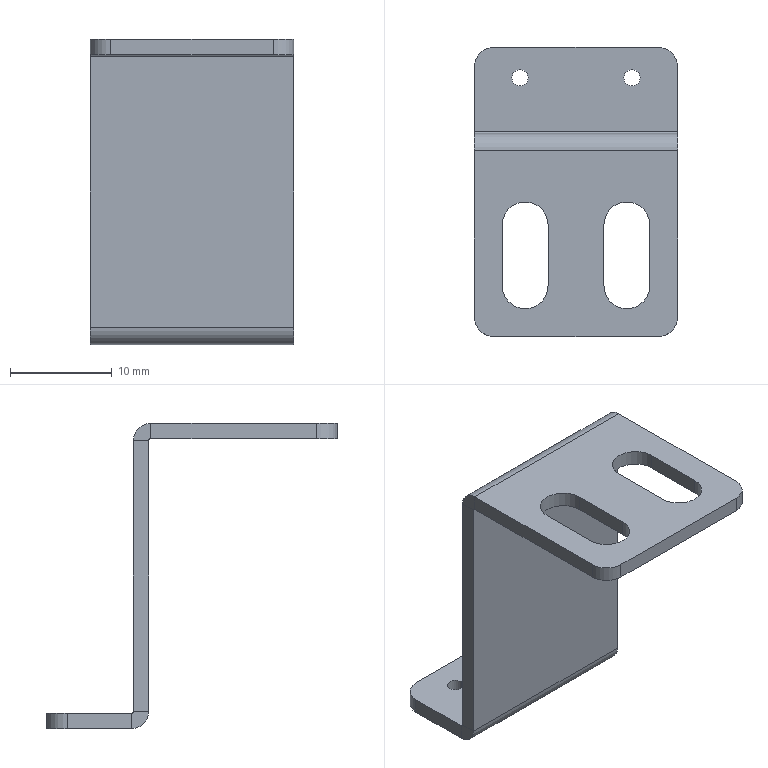Part | STEP file | 1 solid | 38 faces | box 20 x 28.5 x 30 mm | volume 1546 mm3 | plane 22 | cylinder 16 | commonest cylinder face diameters 1.6 x4 4 x4 4.5 x4 0.4 x2 3.4 x2